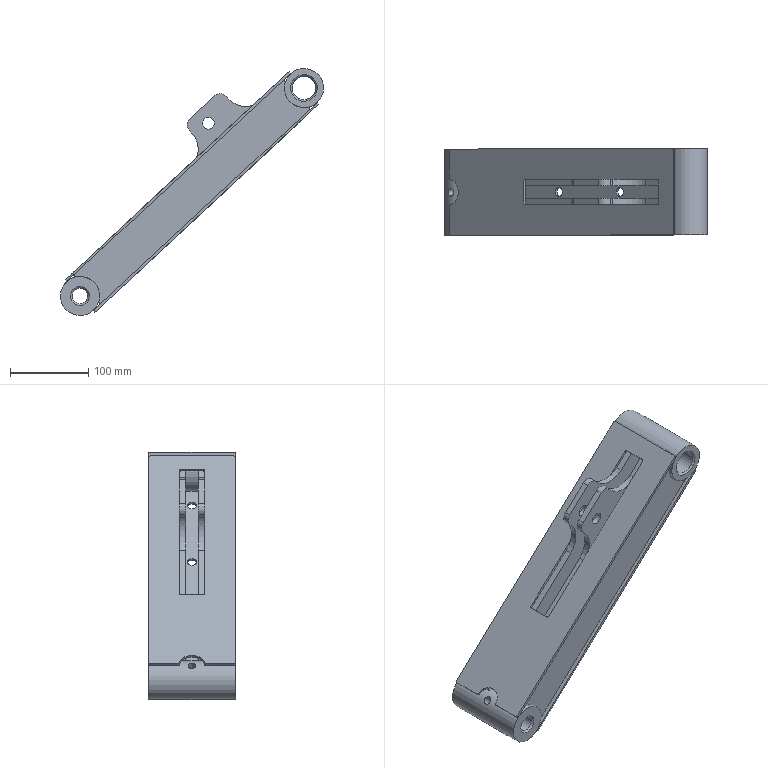Part | STEP file | HL4GZ-1.862.033 (cane-lifter lower swing arm weldment) | 8 solids | 111 faces | box 335.777 x 110 x 315.389 mm | volume 1087087 mm3 | cylinder 60 | plane 47 | cone 4 | commonest cylinder face diameters 4 x30 50 x10 20 x6 12 x4 60 x4 15 x2